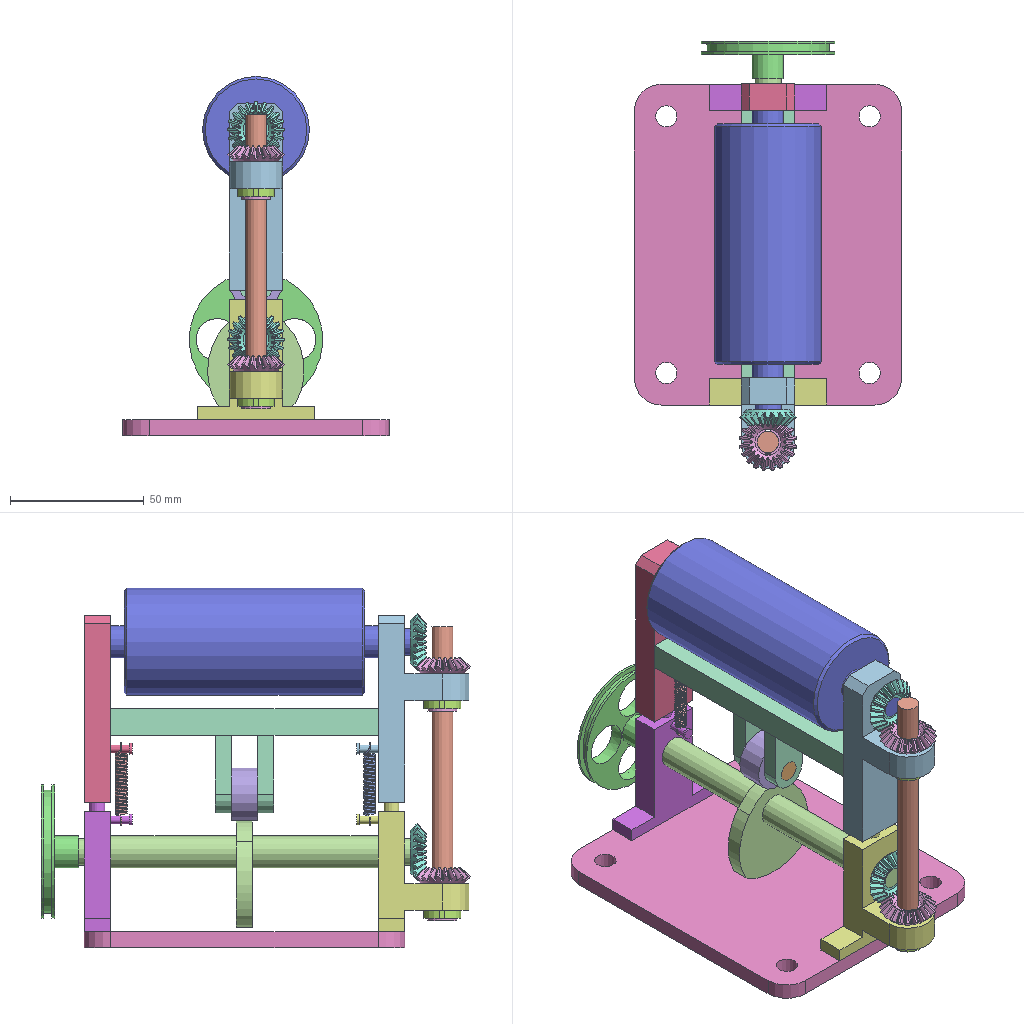Assembly | NX | 16 different items | 19 placed | box 100 x 161 x 134 mm
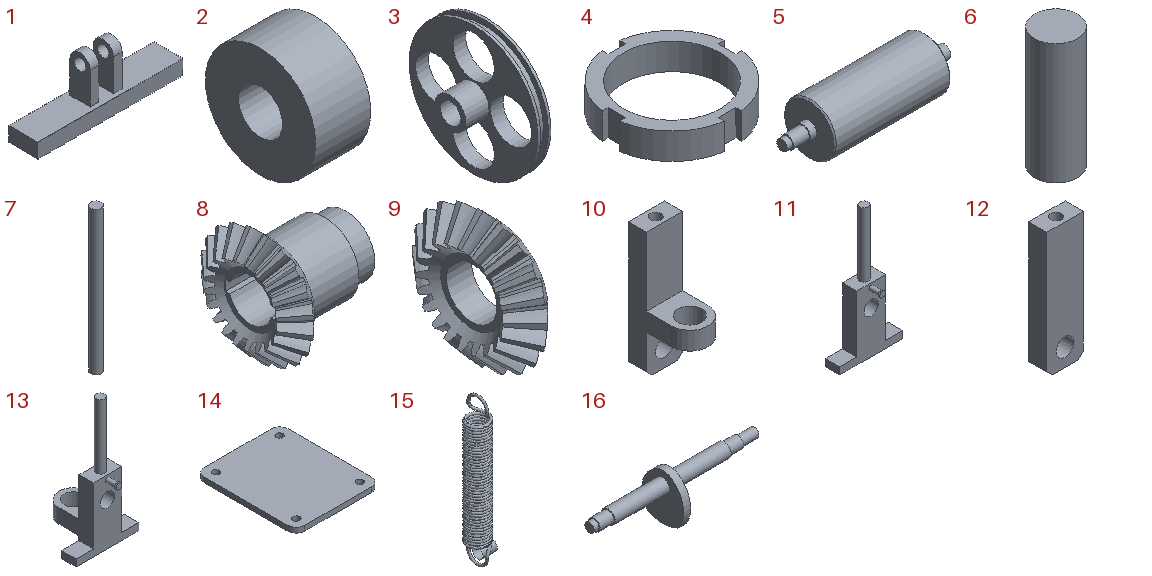Parts list (item | quantity | size | volume | features):
1 | x1 | 100 x 20 x 39 mm | 24046 mm3 | features DATUM_CSYS 2, BLEND 1, BLOCK 1, EXTRUDE 1, HOLE PACKAGE 1, SIMPLE HOLE 1, SKETCH 1
2 | x1 | 10 x 20 x 20 mm | 2639 mm3 | features DATUM_CSYS 2, EXTRUDE 1, SKETCH 1
3 | x1 | 14 x 50 x 50 mm | 5206 mm3 | features DATUM_CSYS 3, SKETCH 2, EXTRUDE 1, SWP104 1
4 | x2 | 13.856 x 13.856 x 3 mm | 159.288 mm3 | features DATUM_CSYS 2, EXTRUDE 1, SKETCH 1
5 | x1 | 126 x 40 x 40 mm | 116034 mm3 | features DATUM_CSYS 2, SKETCH 1, SWP104 1
6 | x1 | 7.8 x 7.8 x 22 mm | 1051 mm3 | features CYLINDER 1, DATUM_CSYS 1
7 | x1 | 8 x 8 x 110 mm | 5529 mm3 | features CYLINDER 1, DATUM_CSYS 1
8 | x2 | 19.993 x 21.268 x 21.268 mm | 1845 mm3 | features EXTRACT_BODY 20, TRIM BODY 20, Instance Feature 19, DATUM_CSYS 3, SKETCH 2, EXTEND_SHEET 1, EXTRUDE 1, Pattern Feature 1, SKIN 1, SWP104 1
9 | x2 | 5.993 x 21.414 x 21.414 mm | 898.737 mm3 | features EXTRACT_BODY 20, TRIM BODY 20, Instance Feature 19, DATUM_CSYS 2, EXTEND_SHEET 1, Pattern Feature 1, SKETCH 1, SKIN 1, SWP104 1
10 | x1 | 20 x 42 x 70 mm | 14816 mm3 | features DATUM_CSYS 5, EXTRUDE 4, SKETCH 4, HOLE PACKAGE 1, SIMPLE HOLE 1
11 | x1 | 44 x 18 x 89.9 mm | 10705 mm3 | features DATUM_CSYS 5, EXTRUDE 4, SKETCH 4
12 | x1 | 20 x 18 x 70 mm | 11773 mm3 | features DATUM_CSYS 4, EXTRUDE 3, SKETCH 3, HOLE PACKAGE 1, SIMPLE HOLE 1
13 | x1 | 44 x 42 x 89.9 mm | 13748 mm3 | features DATUM_CSYS 6, EXTRUDE 5, SKETCH 5
14 | x1 | 100 x 120 x 6 mm | 70279 mm3 | features DATUM_CSYS 2, EXTRUDE 1, SKETCH 1
15 | x1 | 5.249 x 4.5 x 31.219 mm | 113.865 mm3 | features DATUM_CSYS 4, DATUM_AXIS 3, SKETCH 3, BRIDGE_CURVE 2, DATUM_PLANE 2, DATUM_ON_PATH 1, EXTRUDE 1, FLEXIBLE_PART 1, FSET 1, HELIX 1, SKIN 1
16 | x1 | 142 x 36.204 x 40.001 mm | 20323 mm3 | features DATUM_CSYS 2, EXTRUDE 1, SKETCH 1, SWP104 1
Mates (type | each side: item.copy, entity, surface, feature):
Fix | 14.1 component
Touch | 12.1 face plane Extrude(2) | 10.1 face plane Extrude(2) | 2 times
Touch | 1.1 face plane Block(1) | 10.1 face plane Extrude(2)
Touch | 12.1 face plane Extrude(2) | 1.1 face plane Block(1)
Touch | 13.1 face cylinder Extrude(3) | 10.1 face cylinder Ø6 Hole(5)
Touch | 11.1 face cylinder Extrude(3) | 12.1 face cylinder Ø6 Hole(5)
Touch | 13.1 face plane Extrude(2) | 14.1 face plane Extrude(4)
Center22 | 13.1 face plane Extrude(2) | 13.1 face plane Extrude(2) | 14.1 face plane Extrude(4) | 14.1 face plane Extrude(4)
Center22 | 13.1 face plane Extrude(2) | 11.1 face plane Extrude(2) | 14.1 face plane Extrude(4) | 14.1 face plane Extrude(4)
Concentric | 16.1 edge | 13.1 edge
Concentric | 3.1 edge | 16.1 edge
Distance | 10.1 face plane Extrude(2) | 1.1 face plane Block(1)
Concentric | 6.1 edge | 1.1 edge
Concentric | 2.1 edge | 1.1 edge
Touch | 16.1 face swept Extrude(6) | 2.1 face cylinder Extrude(1)
Concentric | 5.1 edge | 10.1 edge
Concentric | 9.1 edge | 5.1 edge
Concentric | 9.1 edge | 16.1 edge
Concentric | 8.1 edge | 10.1 edge
Concentric | 8.1 edge | 13.1 edge
Concentric | 4.1 edge | 8.1 edge | 2 times
Touch | 15.1 face cylinder Extrude(15) | 13.1 face cylinder Extrude(4)
Concentric | 7.1 edge | 8.1 edge